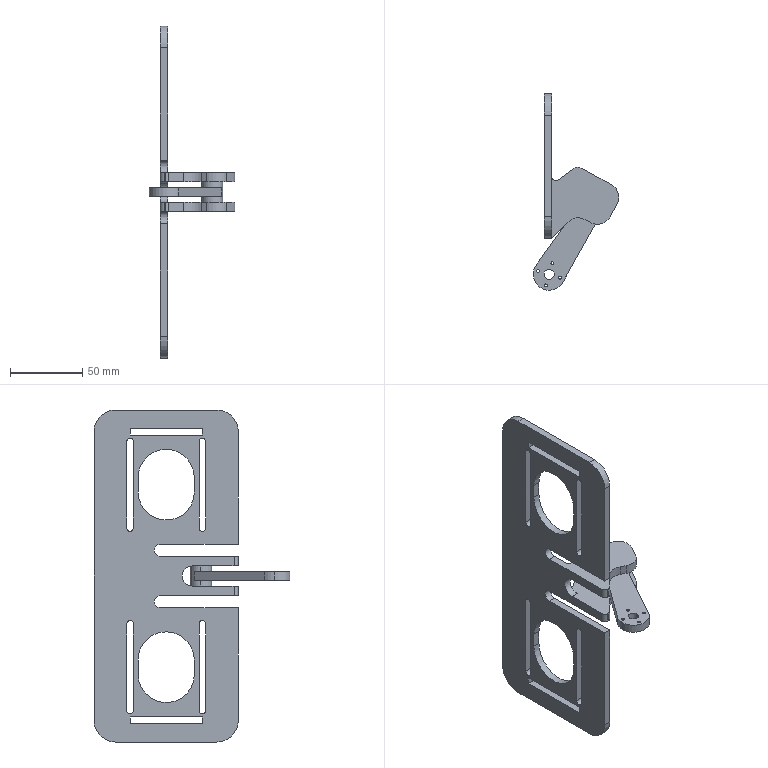Part | SolidWorks | features ICE 12, Cut 3, Fillet 3, MirrorPattern 2, BaseBody 1 | 1 solid | 103 faces | box 59.27 x 135.834 x 230 mm | volume 110956 mm3 | cylinder 54 | plane 49 | commonest cylinder face diameters 4.5 x12 2 x8 20 x7 6 x6 39 x6 30 x4